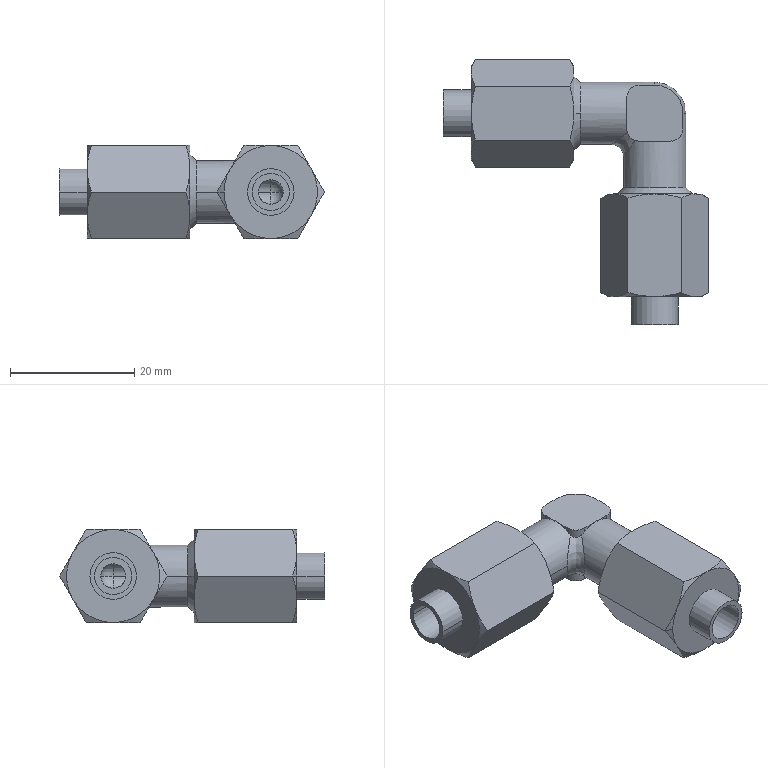Part | SolidWorks | features Boss 5, RevCut 5, Fillet 2, ICE 2, Revolution 2, Sweep 1 | 1 solid | 92 faces | box 42.66 x 42.66 x 15 mm | volume 7800 mm3 | plane 34 | cone 30 | cylinder 24 | sphere 3 | spline 1 | commonest cylinder face diameters 4 x10 6 x4 7.5 x4 10 x4 9 x2